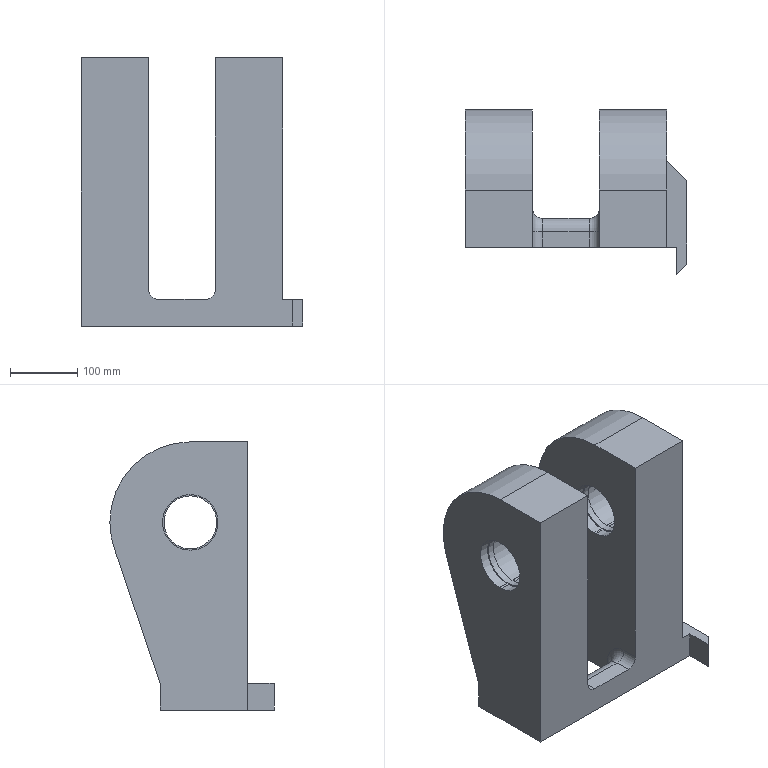Part | NX | features solid 2 | 1 solid | 81 faces | box 330 x 245 x 400 mm | volume 12783624 mm3 | plane 58 | cylinder 21 | torus 2 | commonest cylinder face diameters 83 x12 79 x4 30 x2 240 x2 40 x1